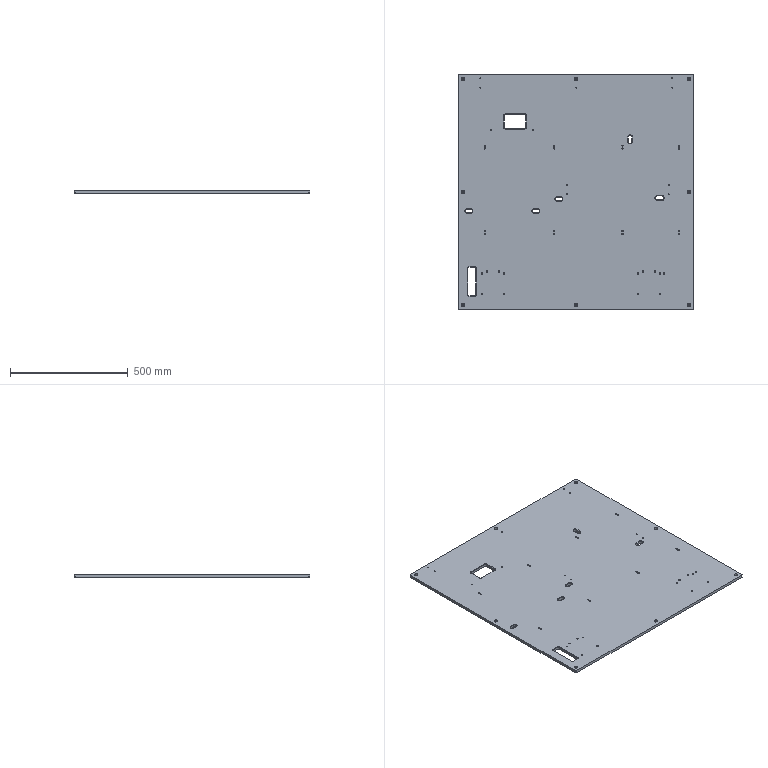Part | STEP file | SynoNew-0304-025 | 1 solid | 151 faces | box 1000 x 1000 x 12 mm | volume 11833739 mm3 | cylinder 78 | plane 55 | cone 18 | commonest cylinder face diameters 5 x24 15 x16 10 x12 4.2 x9 9 x8 6 x5